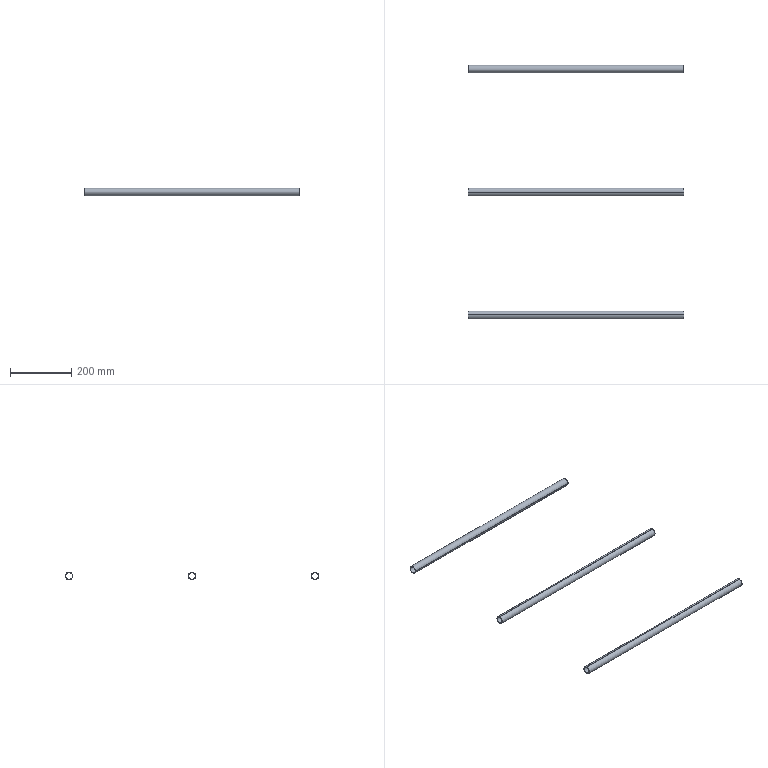Part | STEP file | E3-粉仓护栏10栏杆_Default<As Machined> | 3 solids | 18 faces | box 702.5 x 825 x 25 mm | volume 233387 mm3 | cylinder 12 | plane 6 | commonest cylinder face diameters 22 x6 25 x6
STEP:
#1=CARTESIAN_POINT('',(0.,0.,0.));
#2=DIRECTION('',(0.,0.,1.));
#3=DIRECTION('',(1.,0.,0.));
#4=AXIS2_PLACEMENT_3D('',#1,#2,#3);
#5=CARTESIAN_POINT('',(-702.5,0.,12.5));
#6=VERTEX_POINT('',#5);
#7=CARTESIAN_POINT('',(-702.5,0.,-12.5));
#8=VERTEX_POINT('',#7);
#9=CARTESIAN_POINT('',(-702.5,0.,0.));
#10=DIRECTION('',(1.,0.,0.));
#11=DIRECTION('',(0.,-1.,0.));
#12=AXIS2_PLACEMENT_3D('',#9,#10,#11);
#13=CIRCLE('',#12,12.5);
#14=CARTESIAN_POINT('',(-702.5,0.,0.));
#15=DIRECTION('',(1.,0.,0.));
#16=DIRECTION('',(0.,0.,1.));
#17=AXIS2_PLACEMENT_3D('',#14,#15,#16);
#18=CYLINDRICAL_SURFACE('',#17,12.5);
#19=CARTESIAN_POINT('',(-4.712,0.));
#20=DIRECTION('',(1.,0.));
#21=VECTOR('',#20,1.);
#22=LINE('',#19,#21);
#23=(GEOMETRIC_REPRESENTATION_CONTEXT(2)PARAMETRIC_REPRESENTATION_CONTEXT()REPRESENTATION_CONTEXT('',''));
#24=DEFINITIONAL_REPRESENTATION('',(#22),#23);
#25=PCURVE('',#18,#24);
#26=CARTESIAN_POINT('',(-702.5,0.,0.));
#27=DIRECTION('',(-1.,0.,0.));
#28=DIRECTION('',(0.,-1.,0.));
#29=AXIS2_PLACEMENT_3D('',#26,#27,#28);
#30=PLANE('',#29);
#31=CARTESIAN_POINT('',(12.5,0.));
#32=CARTESIAN_POINT('',(12.5,-21.651));
#33=CARTESIAN_POINT('',(-6.25,-10.825));
#34=CARTESIAN_POINT('',(-25.,0.));
#35=CARTESIAN_POINT('',(-6.25,10.825));
#36=CARTESIAN_POINT('',(12.5,21.651));
#37=CARTESIAN_POINT('',(12.5,0.));
#38=(BOUNDED_CURVE()B_SPLINE_CURVE(2,(#31,#32,#33,#34,#35,#36,#37),.UNSPECIFIED.,.T.,.F.)B_SPLINE_CURVE_WITH_KNOTS((1,2,2,2,2,1),(-2.094,0.,2.094,4.189,6.283,8.378),.UNSPECIFIED.)CURVE()GEOMETRIC_REPRESENTATION_ITEM()RATIONAL_B_SPLINE_CURVE((1.,0.5,1.,0.5,1.,0.5,1.))REPRESENTATION_ITEM(''));
#39=(GEOMETRIC_REPRESENTATION_CONTEXT(2)PARAMETRIC_REPRESENTATION_CONTEXT()REPRESENTATION_CONTEXT('',''));
#40=DEFINITIONAL_REPRESENTATION('',(#38),#39);
#41=PCURVE('',#30,#40);
#42=SURFACE_CURVE('',#13,(#25,#41),.PCURVE_S1.);
#43=EDGE_CURVE('',#6,#8,#42,.T.);
#44=ORIENTED_EDGE('',*,*,#43,.T.);
#45=CARTESIAN_POINT('',(0.,0.,-12.5));
#46=VERTEX_POINT('',#45);
#47=CARTESIAN_POINT('',(-702.5,0.,-12.5));
#48=DIRECTION('',(1.,0.,0.));
#49=VECTOR('',#48,1.);
#50=LINE('',#47,#49);
#51=CARTESIAN_POINT('',(3.142,0.));
#52=DIRECTION('',(0.,1.));
#53=VECTOR('',#52,1.);
#54=LINE('',#51,#53);
#55=(GEOMETRIC_REPRESENTATION_CONTEXT(2)PARAMETRIC_REPRESENTATION_CONTEXT()REPRESENTATION_CONTEXT('',''));
#56=DEFINITIONAL_REPRESENTATION('',(#54),#55);
#57=PCURVE('',#18,#56);
#58=CARTESIAN_POINT('',(-702.5,0.,0.));
#59=DIRECTION('',(1.,0.,0.));
#60=DIRECTION('',(0.,0.,1.));
#61=AXIS2_PLACEMENT_3D('',#58,#59,#60);
#62=CYLINDRICAL_SURFACE('',#61,12.5);
#63=CARTESIAN_POINT('',(3.142,0.));
#64=DIRECTION('',(0.,1.));
#65=VECTOR('',#64,1.);
#66=LINE('',#63,#65);
#67=(GEOMETRIC_REPRESENTATION_CONTEXT(2)PARAMETRIC_REPRESENTATION_CONTEXT()REPRESENTATION_CONTEXT('',''));
#68=DEFINITIONAL_REPRESENTATION('',(#66),#67);
#69=PCURVE('',#62,#68);
#70=SURFACE_CURVE('',#50,(#57,#69),.PCURVE_S1.);
#71=EDGE_CURVE('',#8,#46,#70,.T.);
#72=ORIENTED_EDGE('',*,*,#71,.T.);
#73=CARTESIAN_POINT('',(0.,0.,12.5));
#74=VERTEX_POINT('',#73);
#75=CARTESIAN_POINT('',(0.,0.,0.));
#76=DIRECTION('',(1.,0.,0.));
#77=DIRECTION('',(0.,-1.,0.));
#78=AXIS2_PLACEMENT_3D('',#75,#76,#77);
#79=CIRCLE('',#78,12.5);
#80=CARTESIAN_POINT('',(-4.712,702.5));
#81=DIRECTION('',(1.,0.));
#82=VECTOR('',#81,1.);
#83=LINE('',#80,#82);
#84=(GEOMETRIC_REPRESENTATION_CONTEXT(2)PARAMETRIC_REPRESENTATION_CONTEXT()REPRESENTATION_CONTEXT('',''));
#85=DEFINITIONAL_REPRESENTATION('',(#83),#84);
#86=PCURVE('',#18,#85);
#87=CARTESIAN_POINT('',(0.,0.,0.));
#88=DIRECTION('',(-1.,0.,0.));
#89=DIRECTION('',(0.,-1.,0.));
#90=AXIS2_PLACEMENT_3D('',#87,#88,#89);
#91=PLANE('',#90);
#92=CARTESIAN_POINT('',(12.5,0.));
#93=CARTESIAN_POINT('',(12.5,-21.651));
#94=CARTESIAN_POINT('',(-6.25,-10.825));
#95=CARTESIAN_POINT('',(-25.,0.));
#96=CARTESIAN_POINT('',(-6.25,10.825));
#97=CARTESIAN_POINT('',(12.5,21.651));
#98=CARTESIAN_POINT('',(12.5,0.));
#99=(BOUNDED_CURVE()B_SPLINE_CURVE(2,(#92,#93,#94,#95,#96,#97,#98),.UNSPECIFIED.,.T.,.F.)B_SPLINE_CURVE_WITH_KNOTS((1,2,2,2,2,1),(-2.094,0.,2.094,4.189,6.283,8.378),.UNSPECIFIED.)CURVE()GEOMETRIC_REPRESENTATION_ITEM()RATIONAL_B_SPLINE_CURVE((1.,0.5,1.,0.5,1.,0.5,1.))REPRESENTATION_ITEM(''));
#100=(GEOMETRIC_REPRESENTATION_CONTEXT(2)PARAMETRIC_REPRESENTATION_CONTEXT()REPRESENTATION_CONTEXT('',''));
#101=DEFINITIONAL_REPRESENTATION('',(#99),#100);
#102=PCURVE('',#91,#101);
#103=SURFACE_CURVE('',#79,(#86,#102),.PCURVE_S1.);
#104=EDGE_CURVE('',#74,#46,#103,.T.);
#105=ORIENTED_EDGE('',*,*,#104,.F.);
#106=CARTESIAN_POINT('',(-702.5,0.,12.5));
#107=DIRECTION('',(1.,0.,0.));
#108=VECTOR('',#107,1.);
#109=LINE('',#106,#108);
#110=CARTESIAN_POINT('',(0.,0.));
#111=DIRECTION('',(0.,1.));
#112=VECTOR('',#111,1.);
#113=LINE('',#110,#112);
#114=(GEOMETRIC_REPRESENTATION_CONTEXT(2)PARAMETRIC_REPRESENTATION_CONTEXT()REPRESENTATION_CONTEXT('',''));
#115=DEFINITIONAL_REPRESENTATION('',(#113),#114);
#116=PCURVE('',#18,#115);
#117=CARTESIAN_POINT('',(6.283,0.));
#118=DIRECTION('',(0.,1.));
#119=VECTOR('',#118,1.);
#120=LINE('',#117,#119);
#121=(GEOMETRIC_REPRESENTATION_CONTEXT(2)PARAMETRIC_REPRESENTATION_CONTEXT()REPRESENTATION_CONTEXT('',''));
#122=DEFINITIONAL_REPRESENTATION('',(#120),#121);
#123=PCURVE('',#62,#122);
#124=SURFACE_CURVE('',#109,(#116,#123),.PCURVE_S1.);
#125=EDGE_CURVE('',#6,#74,#124,.T.);
#126=ORIENTED_EDGE('',*,*,#125,.F.);
#127=EDGE_LOOP('',(#44,#72,#105,#126));
#128=FACE_BOUND('',#127,.T.);
#129=ADVANCED_FACE('',(#128),#18,.T.);
#130=CARTESIAN_POINT('',(-702.5,0.,11.));
#131=VERTEX_POINT('',#130);
#132=CARTESIAN_POINT('',(0.,0.,11.));
#133=VERTEX_POINT('',#132);
#134=CARTESIAN_POINT('',(-702.5,0.,11.));
#135=DIRECTION('',(1.,0.,0.));
#136=VECTOR('',#135,1.);
#137=LINE('',#134,#136);
#138=CARTESIAN_POINT('',(-702.5,0.,0.));
#139=DIRECTION('',(1.,0.,0.));
#140=DIRECTION('',(0.,0.,1.));
#141=AXIS2_PLACEMENT_3D('',#138,#139,#140);
#142=CYLINDRICAL_SURFACE('',#141,11.);
#143=CARTESIAN_POINT('',(6.283,0.));
#144=DIRECTION('',(0.,1.));
#145=VECTOR('',#144,1.);
#146=LINE('',#143,#145);
#147=(GEOMETRIC_REPRESENTATION_CONTEXT(2)PARAMETRIC_REPRESENTATION_CONTEXT()REPRESENTATION_CONTEXT('',''));
#148=DEFINITIONAL_REPRESENTATION('',(#146),#147);
#149=PCURVE('',#142,#148);
#150=CARTESIAN_POINT('',(-702.5,0.,0.));
#151=DIRECTION('',(1.,0.,0.));
#152=DIRECTION('',(0.,0.,1.));
#153=AXIS2_PLACEMENT_3D('',#150,#151,#152);
#154=CYLINDRICAL_SURFACE('',#153,11.);
#155=CARTESIAN_POINT('',(0.,0.));
#156=DIRECTION('',(0.,1.));
#157=VECTOR('',#156,1.);
#158=LINE('',#155,#157);
#159=(GEOMETRIC_REPRESENTATION_CONTEXT(2)PARAMETRIC_REPRESENTATION_CONTEXT()REPRESENTATION_CONTEXT('',''));
#160=DEFINITIONAL_REPRESENTATION('',(#158),#159);
#161=PCURVE('',#154,#160);
#162=SURFACE_CURVE('',#137,(#149,#161),.PCURVE_S1.);
#163=EDGE_CURVE('',#131,#133,#162,.T.);
#164=ORIENTED_EDGE('',*,*,#163,.T.);
#165=CARTESIAN_POINT('',(0.,0.,-11.));
#166=VERTEX_POINT('',#165);
#167=CARTESIAN_POINT('',(0.,0.,0.));
#168=DIRECTION('',(1.,0.,0.));
#169=DIRECTION('',(0.,-1.,0.));
#170=AXIS2_PLACEMENT_3D('',#167,#168,#169);
#171=CIRCLE('',#170,11.);
#172=CARTESIAN_POINT('',(1.571,702.5));
#173=DIRECTION('',(1.,0.));
#174=VECTOR('',#173,1.);
#175=LINE('',#172,#174);
#176=(GEOMETRIC_REPRESENTATION_CONTEXT(2)PARAMETRIC_REPRESENTATION_CONTEXT()REPRESENTATION_CONTEXT('',''));
#177=DEFINITIONAL_REPRESENTATION('',(#175),#176);
#178=PCURVE('',#142,#177);
#179=CARTESIAN_POINT('',(11.,0.));
#180=CARTESIAN_POINT('',(11.,-19.053));
#181=CARTESIAN_POINT('',(-5.5,-9.526));
#182=CARTESIAN_POINT('',(-22.,0.));
#183=CARTESIAN_POINT('',(-5.5,9.526));
#184=CARTESIAN_POINT('',(11.,19.053));
#185=CARTESIAN_POINT('',(11.,0.));
#186=(BOUNDED_CURVE()B_SPLINE_CURVE(2,(#179,#180,#181,#182,#183,#184,#185),.UNSPECIFIED.,.T.,.F.)B_SPLINE_CURVE_WITH_KNOTS((1,2,2,2,2,1),(-2.094,0.,2.094,4.189,6.283,8.378),.UNSPECIFIED.)CURVE()GEOMETRIC_REPRESENTATION_ITEM()RATIONAL_B_SPLINE_CURVE((1.,0.5,1.,0.5,1.,0.5,1.))REPRESENTATION_ITEM(''));
#187=(GEOMETRIC_REPRESENTATION_CONTEXT(2)PARAMETRIC_REPRESENTATION_CONTEXT()REPRESENTATION_CONTEXT('',''));
#188=DEFINITIONAL_REPRESENTATION('',(#186),#187);
#189=PCURVE('',#91,#188);
#190=SURFACE_CURVE('',#171,(#178,#189),.PCURVE_S1.);
#191=EDGE_CURVE('',#166,#133,#190,.T.);
#192=ORIENTED_EDGE('',*,*,#191,.F.);
#193=CARTESIAN_POINT('',(-702.5,0.,-11.));
#194=VERTEX_POINT('',#193);
#195=CARTESIAN_POINT('',(-702.5,0.,-11.));
#196=DIRECTION('',(1.,0.,0.));
#197=VECTOR('',#196,1.);
#198=LINE('',#195,#197);
#199=CARTESIAN_POINT('',(3.142,0.));
#200=DIRECTION('',(0.,1.));
#201=VECTOR('',#200,1.);
#202=LINE('',#199,#201);
#203=(GEOMETRIC_REPRESENTATION_CONTEXT(2)PARAMETRIC_REPRESENTATION_CONTEXT()REPRESENTATION_CONTEXT('',''));
#204=DEFINITIONAL_REPRESENTATION('',(#202),#203);
#205=PCURVE('',#142,#204);
#206=CARTESIAN_POINT('',(3.142,0.));
#207=DIRECTION('',(0.,1.));
#208=VECTOR('',#207,1.);
#209=LINE('',#206,#208);
#210=(GEOMETRIC_REPRESENTATION_CONTEXT(2)PARAMETRIC_REPRESENTATION_CONTEXT()REPRESENTATION_CONTEXT('',''));
#211=DEFINITIONAL_REPRESENTATION('',(#209),#210);
#212=PCURVE('',#154,#211);
#213=SURFACE_CURVE('',#198,(#205,#212),.PCURVE_S1.);
#214=EDGE_CURVE('',#194,#166,#213,.T.);
#215=ORIENTED_EDGE('',*,*,#214,.F.);
#216=CARTESIAN_POINT('',(-702.5,0.,0.));
#217=DIRECTION('',(1.,0.,0.));
#218=DIRECTION('',(0.,-1.,0.));
#219=AXIS2_PLACEMENT_3D('',#216,#217,#218);
#220=CIRCLE('',#219,11.);
#221=CARTESIAN_POINT('',(1.571,0.));
#222=DIRECTION('',(1.,0.));
#223=VECTOR('',#222,1.);
#224=LINE('',#221,#223);
#225=(GEOMETRIC_REPRESENTATION_CONTEXT(2)PARAMETRIC_REPRESENTATION_CONTEXT()REPRESENTATION_CONTEXT('',''));
#226=DEFINITIONAL_REPRESENTATION('',(#224),#225);
#227=PCURVE('',#142,#226);
#228=CARTESIAN_POINT('',(11.,0.));
#229=CARTESIAN_POINT('',(11.,-19.053));
#230=CARTESIAN_POINT('',(-5.5,-9.526));
#231=CARTESIAN_POINT('',(-22.,0.));
#232=CARTESIAN_POINT('',(-5.5,9.526));
#233=CARTESIAN_POINT('',(11.,19.053));
#234=CARTESIAN_POINT('',(11.,0.));
#235=(BOUNDED_CURVE()B_SPLINE_CURVE(2,(#228,#229,#230,#231,#232,#233,#234),.UNSPECIFIED.,.T.,.F.)B_SPLINE_CURVE_WITH_KNOTS((1,2,2,2,2,1),(-2.094,0.,2.094,4.189,6.283,8.378),.UNSPECIFIED.)CURVE()GEOMETRIC_REPRESENTATION_ITEM()RATIONAL_B_SPLINE_CURVE((1.,0.5,1.,0.5,1.,0.5,1.))REPRESENTATION_ITEM(''));
#236=(GEOMETRIC_REPRESENTATION_CONTEXT(2)PARAMETRIC_REPRESENTATION_CONTEXT()REPRESENTATION_CONTEXT('',''));
#237=DEFINITIONAL_REPRESENTATION('',(#235),#236);
#238=PCURVE('',#30,#237);
#239=SURFACE_CURVE('',#220,(#227,#238),.PCURVE_S1.);
#240=EDGE_CURVE('',#194,#131,#239,.T.);
#241=ORIENTED_EDGE('',*,*,#240,.T.);
#242=EDGE_LOOP('',(#164,#192,#215,#241));
#243=FACE_BOUND('',#242,.F.);
#244=ADVANCED_FACE('',(#243),#142,.F.);
#245=CARTESIAN_POINT('',(0.,0.,0.));
#246=DIRECTION('',(1.,0.,0.));
#247=DIRECTION('',(0.,-1.,0.));
#248=AXIS2_PLACEMENT_3D('',#245,#246,#247);
#249=CIRCLE('',#248,11.);
#250=CARTESIAN_POINT('',(-4.712,702.5));
#251=DIRECTION('',(1.,0.));
#252=VECTOR('',#251,1.);
#253=LINE('',#250,#252);
#254=(GEOMETRIC_REPRESENTATION_CONTEXT(2)PARAMETRIC_REPRESENTATION_CONTEXT()REPRESENTATION_CONTEXT('',''));
#255=DEFINITIONAL_REPRESENTATION('',(#253),#254);
#256=PCURVE('',#154,#255);
#257=CARTESIAN_POINT('',(11.,0.));
#258=CARTESIAN_POINT('',(11.,-19.053));
#259=CARTESIAN_POINT('',(-5.5,-9.526));
#260=CARTESIAN_POINT('',(-22.,0.));
#261=CARTESIAN_POINT('',(-5.5,9.526));
#262=CARTESIAN_POINT('',(11.,19.053));
#263=CARTESIAN_POINT('',(11.,0.));
#264=(BOUNDED_CURVE()B_SPLINE_CURVE(2,(#257,#258,#259,#260,#261,#262,#263),.UNSPECIFIED.,.T.,.F.)B_SPLINE_CURVE_WITH_KNOTS((1,2,2,2,2,1),(-2.094,0.,2.094,4.189,6.283,8.378),.UNSPECIFIED.)CURVE()GEOMETRIC_REPRESENTATION_ITEM()RATIONAL_B_SPLINE_CURVE((1.,0.5,1.,0.5,1.,0.5,1.))REPRESENTATION_ITEM(''));
#265=(GEOMETRIC_REPRESENTATION_CONTEXT(2)PARAMETRIC_REPRESENTATION_CONTEXT()REPRESENTATION_CONTEXT('',''));
#266=DEFINITIONAL_REPRESENTATION('',(#264),#265);
#267=PCURVE('',#91,#266);
#268=SURFACE_CURVE('',#249,(#256,#267),.PCURVE_S1.);
#269=EDGE_CURVE('',#133,#166,#268,.T.);
#270=ORIENTED_EDGE('',*,*,#269,.F.);
#271=ORIENTED_EDGE('',*,*,#163,.F.);
#272=CARTESIAN_POINT('',(-702.5,0.,0.));
#273=DIRECTION('',(1.,0.,0.));
#274=DIRECTION('',(0.,-1.,0.));
#275=AXIS2_PLACEMENT_3D('',#272,#273,#274);
#276=CIRCLE('',#275,11.);
#277=CARTESIAN_POINT('',(-4.712,0.));
#278=DIRECTION('',(1.,0.));
#279=VECTOR('',#278,1.);
#280=LINE('',#277,#279);
#281=(GEOMETRIC_REPRESENTATION_CONTEXT(2)PARAMETRIC_REPRESENTATION_CONTEXT()REPRESENTATION_CONTEXT('',''));
#282=DEFINITIONAL_REPRESENTATION('',(#280),#281);
#283=PCURVE('',#154,#282);
#284=CARTESIAN_POINT('',(11.,0.));
#285=CARTESIAN_POINT('',(11.,-19.053));
#286=CARTESIAN_POINT('',(-5.5,-9.526));
#287=CARTESIAN_POINT('',(-22.,0.));
#288=CARTESIAN_POINT('',(-5.5,9.526));
#289=CARTESIAN_POINT('',(11.,19.053));
#290=CARTESIAN_POINT('',(11.,0.));
#291=(BOUNDED_CURVE()B_SPLINE_CURVE(2,(#284,#285,#286,#287,#288,#289,#290),.UNSPECIFIED.,.T.,.F.)B_SPLINE_CURVE_WITH_KNOTS((1,2,2,2,2,1),(-2.094,0.,2.094,4.189,6.283,8.378),.UNSPECIFIED.)CURVE()GEOMETRIC_REPRESENTATION_ITEM()RATIONAL_B_SPLINE_CURVE((1.,0.5,1.,0.5,1.,0.5,1.))REPRESENTATION_ITEM(''));
#292=(GEOMETRIC_REPRESENTATION_CONTEXT(2)PARAMETRIC_REPRESENTATION_CONTEXT()REPRESENTATION_CONTEXT('',''));
#293=DEFINITIONAL_REPRESENTATION('',(#291),#292);
#294=PCURVE('',#30,#293);
#295=SURFACE_CURVE('',#276,(#283,#294),.PCURVE_S1.);
#296=EDGE_CURVE('',#131,#194,#295,.T.);
#297=ORIENTED_EDGE('',*,*,#296,.T.);
#298=ORIENTED_EDGE('',*,*,#214,.T.);
#299=EDGE_LOOP('',(#270,#271,#297,#298));
#300=FACE_BOUND('',#299,.F.);
#301=ADVANCED_FACE('',(#300),#154,.F.);
#302=ORIENTED_EDGE('',*,*,#71,.F.);
#303=CARTESIAN_POINT('',(-702.5,0.,0.));
#304=DIRECTION('',(1.,0.,0.));
#305=DIRECTION('',(0.,-1.,0.));
#306=AXIS2_PLACEMENT_3D('',#303,#304,#305);
#307=CIRCLE('',#306,12.5);
#308=CARTESIAN_POINT('',(1.571,0.));
#309=DIRECTION('',(1.,0.));
#310=VECTOR('',#309,1.);
#311=LINE('',#308,#310);
#312=(GEOMETRIC_REPRESENTATION_CONTEXT(2)PARAMETRIC_REPRESENTATION_CONTEXT()REPRESENTATION_CONTEXT('',''));
#313=DEFINITIONAL_REPRESENTATION('',(#311),#312);
#314=PCURVE('',#62,#313);
#315=CARTESIAN_POINT('',(12.5,0.));
#316=CARTESIAN_POINT('',(12.5,-21.651));
#317=CARTESIAN_POINT('',(-6.25,-10.825));
#318=CARTESIAN_POINT('',(-25.,0.));
#319=CARTESIAN_POINT('',(-6.25,10.825));
#320=CARTESIAN_POINT('',(12.5,21.651));
#321=CARTESIAN_POINT('',(12.5,0.));
#322=(BOUNDED_CURVE()B_SPLINE_CURVE(2,(#315,#316,#317,#318,#319,#320,#321),.UNSPECIFIED.,.T.,.F.)B_SPLINE_CURVE_WITH_KNOTS((1,2,2,2,2,1),(-2.094,0.,2.094,4.189,6.283,8.378),.UNSPECIFIED.)CURVE()GEOMETRIC_REPRESENTATION_ITEM()RATIONAL_B_SPLINE_CURVE((1.,0.5,1.,0.5,1.,0.5,1.))REPRESENTATION_ITEM(''));
#323=(GEOMETRIC_REPRESENTATION_CONTEXT(2)PARAMETRIC_REPRESENTATION_CONTEXT()REPRESENTATION_CONTEXT('',''));
#324=DEFINITIONAL_REPRESENTATION('',(#322),#323);
#325=PCURVE('',#30,#324);
#326=SURFACE_CURVE('',#307,(#314,#325),.PCURVE_S1.);
#327=EDGE_CURVE('',#8,#6,#326,.T.);
#328=ORIENTED_EDGE('',*,*,#327,.T.);
#329=ORIENTED_EDGE('',*,*,#125,.T.);
#330=CARTESIAN_POINT('',(0.,0.,0.));
#331=DIRECTION('',(1.,0.,0.));
#332=DIRECTION('',(0.,-1.,0.));
#333=AXIS2_PLACEMENT_3D('',#330,#331,#332);
#334=CIRCLE('',#333,12.5);
#335=CARTESIAN_POINT('',(1.571,702.5));
#336=DIRECTION('',(1.,0.));
#337=VECTOR('',#336,1.);
#338=LINE('',#335,#337);
#339=(GEOMETRIC_REPRESENTATION_CONTEXT(2)PARAMETRIC_REPRESENTATION_CONTEXT()REPRESENTATION_CONTEXT('',''));
#340=DEFINITIONAL_REPRESENTATION('',(#338),#339);
#341=PCURVE('',#62,#340);
#342=CARTESIAN_POINT('',(12.5,0.));
#343=CARTESIAN_POINT('',(12.5,-21.651));
#344=CARTESIAN_POINT('',(-6.25,-10.825));
#345=CARTESIAN_POINT('',(-25.,0.));
#346=CARTESIAN_POINT('',(-6.25,10.825));
#347=CARTESIAN_POINT('',(12.5,21.651));
#348=CARTESIAN_POINT('',(12.5,0.));
#349=(BOUNDED_CURVE()B_SPLINE_CURVE(2,(#342,#343,#344,#345,#346,#347,#348),.UNSPECIFIED.,.T.,.F.)B_SPLINE_CURVE_WITH_KNOTS((1,2,2,2,2,1),(-2.094,0.,2.094,4.189,6.283,8.378),.UNSPECIFIED.)CURVE()GEOMETRIC_REPRESENTATION_ITEM()RATIONAL_B_SPLINE_CURVE((1.,0.5,1.,0.5,1.,0.5,1.))REPRESENTATION_ITEM(''));
#350=(GEOMETRIC_REPRESENTATION_CONTEXT(2)PARAMETRIC_REPRESENTATION_CONTEXT()REPRESENTATION_CONTEXT('',''));
#351=DEFINITIONAL_REPRESENTATION('',(#349),#350);
#352=PCURVE('',#91,#351);
#353=SURFACE_CURVE('',#334,(#341,#352),.PCURVE_S1.);
#354=EDGE_CURVE('',#46,#74,#353,.T.);
#355=ORIENTED_EDGE('',*,*,#354,.F.);
#356=EDGE_LOOP('',(#302,#328,#329,#355));
#357=FACE_BOUND('',#356,.T.);
#358=ADVANCED_FACE('',(#357),#62,.T.);
#359=ORIENTED_EDGE('',*,*,#296,.T.);
#360=ORIENTED_EDGE('',*,*,#240,.T.);
#361=EDGE_LOOP('',(#359,#360));
#362=FACE_BOUND('',#361,.T.);
#363=ORIENTED_EDGE('',*,*,#43,.F.);
#364=ORIENTED_EDGE('',*,*,#327,.F.);
#365=EDGE_LOOP('',(#363,#364));
#366=FACE_BOUND('',#365,.T.);
#367=ADVANCED_FACE('',(#362,#366),#30,.T.);
#368=ORIENTED_EDGE('',*,*,#269,.F.);
#369=ORIENTED_EDGE('',*,*,#191,.F.);
#370=EDGE_LOOP('',(#368,#369));
#371=FACE_BOUND('',#370,.T.);
#372=ORIENTED_EDGE('',*,*,#104,.T.);
#373=ORIENTED_EDGE('',*,*,#354,.T.);
#374=EDGE_LOOP('',(#372,#373));
#375=FACE_BOUND('',#374,.T.);
#376=ADVANCED_FACE('',(#371,#375),#91,.F.);
#377=CLOSED_SHELL('',(#129,#244,#301,#358,#367,#376));
#378=MANIFOLD_SOLID_BREP('',#377);
#379=CARTESIAN_POINT('',(-702.5,812.5,0.));
#380=VERTEX_POINT('',#379);
#381=CARTESIAN_POINT('',(-702.5,787.5,0.));
#382=VERTEX_POINT('',#381);
#383=CARTESIAN_POINT('',(-702.5,800.,0.));
#384=DIRECTION('',(1.,0.,0.));
#385=DIRECTION('',(0.,-1.,0.));
#386=AXIS2_PLACEMENT_3D('',#383,#384,#385);
#387=CIRCLE('',#386,12.5);
#388=CARTESIAN_POINT('',(-702.5,800.,0.));
#389=DIRECTION('',(1.,0.,0.));
#390=DIRECTION('',(0.,1.,0.));
#391=AXIS2_PLACEMENT_3D('',#388,#389,#390);
#392=CYLINDRICAL_SURFACE('',#391,12.5);
#393=CARTESIAN_POINT('',(-3.142,0.));
#394=DIRECTION('',(1.,0.));
#395=VECTOR('',#394,1.);
#396=LINE('',#393,#395);
#397=(GEOMETRIC_REPRESENTATION_CONTEXT(2)PARAMETRIC_REPRESENTATION_CONTEXT()REPRESENTATION_CONTEXT('',''));
#398=DEFINITIONAL_REPRESENTATION('',(#396),#397);
#399=PCURVE('',#392,#398);
#400=CARTESIAN_POINT('',(-702.5,800.,0.));
#401=DIRECTION('',(-1.,0.,0.));
#402=DIRECTION('',(0.,-1.,0.));
#403=AXIS2_PLACEMENT_3D('',#400,#401,#402);
#404=PLANE('',#403);
#405=CARTESIAN_POINT('',(12.5,0.));
#406=CARTESIAN_POINT('',(12.5,-21.651));
#407=CARTESIAN_POINT('',(-6.25,-10.825));
#408=CARTESIAN_POINT('',(-25.,0.));
#409=CARTESIAN_POINT('',(-6.25,10.825));
#410=CARTESIAN_POINT('',(12.5,21.651));
#411=CARTESIAN_POINT('',(12.5,0.));
#412=(BOUNDED_CURVE()B_SPLINE_CURVE(2,(#405,#406,#407,#408,#409,#410,#411),.UNSPECIFIED.,.T.,.F.)B_SPLINE_CURVE_WITH_KNOTS((1,2,2,2,2,1),(-2.094,0.,2.094,4.189,6.283,8.378),.UNSPECIFIED.)CURVE()GEOMETRIC_REPRESENTATION_ITEM()RATIONAL_B_SPLINE_CURVE((1.,0.5,1.,0.5,1.,0.5,1.))REPRESENTATION_ITEM(''));
#413=(GEOMETRIC_REPRESENTATION_CONTEXT(2)PARAMETRIC_REPRESENTATION_CONTEXT()REPRESENTATION_CONTEXT('',''));
#414=DEFINITIONAL_REPRESENTATION('',(#412),#413);
#415=PCURVE('',#404,#414);
#416=SURFACE_CURVE('',#387,(#399,#415),.PCURVE_S1.);
#417=EDGE_CURVE('',#380,#382,#416,.T.);
#418=ORIENTED_EDGE('',*,*,#417,.T.);
#419=CARTESIAN_POINT('',(0.,787.5,0.));
#420=VERTEX_POINT('',#419);
#421=CARTESIAN_POINT('',(-702.5,787.5,0.));
#422=DIRECTION('',(1.,0.,0.));
#423=VECTOR('',#422,1.);
#424=LINE('',#421,#423);
#425=CARTESIAN_POINT('',(3.142,0.));
#426=DIRECTION('',(0.,1.));
#427=VECTOR('',#426,1.);
#428=LINE('',#425,#427);
#429=(GEOMETRIC_REPRESENTATION_CONTEXT(2)PARAMETRIC_REPRESENTATION_CONTEXT()REPRESENTATION_CONTEXT('',''));
#430=DEFINITIONAL_REPRESENTATION('',(#428),#429);
#431=PCURVE('',#392,#430);
#432=CARTESIAN_POINT('',(-702.5,800.,0.));
#433=DIRECTION('',(1.,0.,0.));
#434=DIRECTION('',(0.,1.,0.));
#435=AXIS2_PLACEMENT_3D('',#432,#433,#434);
#436=CYLINDRICAL_SURFACE('',#435,12.5);
#437=CARTESIAN_POINT('',(3.142,0.));
#438=DIRECTION('',(0.,1.));
#439=VECTOR('',#438,1.);
#440=LINE('',#437,#439);
#441=(GEOMETRIC_REPRESENTATION_CONTEXT(2)PARAMETRIC_REPRESENTATION_CONTEXT()REPRESENTATION_CONTEXT('',''));
#442=DEFINITIONAL_REPRESENTATION('',(#440),#441);
#443=PCURVE('',#436,#442);
#444=SURFACE_CURVE('',#424,(#431,#443),.PCURVE_S1.);
#445=EDGE_CURVE('',#382,#420,#444,.T.);
#446=ORIENTED_EDGE('',*,*,#445,.T.);
#447=CARTESIAN_POINT('',(0.,812.5,0.));
#448=VERTEX_POINT('',#447);
#449=CARTESIAN_POINT('',(0.,800.,0.));
#450=DIRECTION('',(1.,0.,0.));
#451=DIRECTION('',(0.,-1.,0.));
#452=AXIS2_PLACEMENT_3D('',#449,#450,#451);
#453=CIRCLE('',#452,12.5);
#454=CARTESIAN_POINT('',(-3.142,702.5));
#455=DIRECTION('',(1.,0.));
#456=VECTOR('',#455,1.);
#457=LINE('',#454,#456);
#458=(GEOMETRIC_REPRESENTATION_CONTEXT(2)PARAMETRIC_REPRESENTATION_CONTEXT()REPRESENTATION_CONTEXT('',''));
#459=DEFINITIONAL_REPRESENTATION('',(#457),#458);
#460=PCURVE('',#392,#459);
#461=CARTESIAN_POINT('',(0.,800.,0.));
#462=DIRECTION('',(-1.,0.,0.));
#463=DIRECTION('',(0.,-1.,0.));
#464=AXIS2_PLACEMENT_3D('',#461,#462,#463);
#465=PLANE('',#464);
#466=CARTESIAN_POINT('',(12.5,0.));
#467=CARTESIAN_POINT('',(12.5,-21.651));
#468=CARTESIAN_POINT('',(-6.25,-10.825));
#469=CARTESIAN_POINT('',(-25.,0.));
#470=CARTESIAN_POINT('',(-6.25,10.825));
#471=CARTESIAN_POINT('',(12.5,21.651));
#472=CARTESIAN_POINT('',(12.5,0.));
#473=(BOUNDED_CURVE()B_SPLINE_CURVE(2,(#466,#467,#468,#469,#470,#471,#472),.UNSPECIFIED.,.T.,.F.)B_SPLINE_CURVE_WITH_KNOTS((1,2,2,2,2,1),(-2.094,0.,2.094,4.189,6.283,8.378),.UNSPECIFIED.)CURVE()GEOMETRIC_REPRESENTATION_ITEM()RATIONAL_B_SPLINE_CURVE((1.,0.5,1.,0.5,1.,0.5,1.))REPRESENTATION_ITEM(''));
#474=(GEOMETRIC_REPRESENTATION_CONTEXT(2)PARAMETRIC_REPRESENTATION_CONTEXT()REPRESENTATION_CONTEXT('',''));
#475=DEFINITIONAL_REPRESENTATION('',(#473),#474);
#476=PCURVE('',#465,#475);
#477=SURFACE_CURVE('',#453,(#460,#476),.PCURVE_S1.);
#478=EDGE_CURVE('',#448,#420,#477,.T.);
#479=ORIENTED_EDGE('',*,*,#478,.F.);
#480=CARTESIAN_POINT('',(-702.5,812.5,0.));
#481=DIRECTION('',(1.,0.,0.));
#482=VECTOR('',#481,1.);
#483=LINE('',#480,#482);
#484=CARTESIAN_POINT('',(0.,0.));
#485=DIRECTION('',(0.,1.));
#486=VECTOR('',#485,1.);
#487=LINE('',#484,#486);
#488=(GEOMETRIC_REPRESENTATION_CONTEXT(2)PARAMETRIC_REPRESENTATION_CONTEXT()REPRESENTATION_CONTEXT('',''));
#489=DEFINITIONAL_REPRESENTATION('',(#487),#488);
#490=PCURVE('',#392,#489);
#491=CARTESIAN_POINT('',(6.283,0.));
#492=DIRECTION('',(0.,1.));
#493=VECTOR('',#492,1.);
#494=LINE('',#491,#493);
#495=(GEOMETRIC_REPRESENTATION_CONTEXT(2)PARAMETRIC_REPRESENTATION_CONTEXT()REPRESENTATION_CONTEXT('',''));
#496=DEFINITIONAL_REPRESENTATION('',(#494),#495);
#497=PCURVE('',#436,#496);
#498=SURFACE_CURVE('',#483,(#490,#497),.PCURVE_S1.);
#499=EDGE_CURVE('',#380,#448,#498,.T.);
#500=ORIENTED_EDGE('',*,*,#499,.F.);
#501=EDGE_LOOP('',(#418,#446,#479,#500));
#502=FACE_BOUND('',#501,.T.);
#503=ADVANCED_FACE('',(#502),#392,.T.);
#504=CARTESIAN_POINT('',(-702.5,811.,0.));
#505=VERTEX_POINT('',#504);
#506=CARTESIAN_POINT('',(0.,811.,0.));
#507=VERTEX_POINT('',#506);
#508=CARTESIAN_POINT('',(-702.5,811.,0.));
#509=DIRECTION('',(1.,0.,0.));
#510=VECTOR('',#509,1.);
#511=LINE('',#508,#510);
#512=CARTESIAN_POINT('',(-702.5,800.,0.));
#513=DIRECTION('',(1.,0.,0.));
#514=DIRECTION('',(0.,1.,0.));
#515=AXIS2_PLACEMENT_3D('',#512,#513,#514);
#516=CYLINDRICAL_SURFACE('',#515,11.);
#517=CARTESIAN_POINT('',(6.283,0.));
#518=DIRECTION('',(0.,1.));
#519=VECTOR('',#518,1.);
#520=LINE('',#517,#519);
#521=(GEOMETRIC_REPRESENTATION_CONTEXT(2)PARAMETRIC_REPRESENTATION_CONTEXT()REPRESENTATION_CONTEXT('',''));
#522=DEFINITIONAL_REPRESENTATION('',(#520),#521);
#523=PCURVE('',#516,#522);
#524=CARTESIAN_POINT('',(-702.5,800.,0.));
#525=DIRECTION('',(1.,0.,0.));
#526=DIRECTION('',(0.,1.,0.));
#527=AXIS2_PLACEMENT_3D('',#524,#525,#526);
#528=CYLINDRICAL_SURFACE('',#527,11.);
#529=CARTESIAN_POINT('',(0.,0.));
#530=DIRECTION('',(0.,1.));
#531=VECTOR('',#530,1.);
#532=LINE('',#529,#531);
#533=(GEOMETRIC_REPRESENTATION_CONTEXT(2)PARAMETRIC_REPRESENTATION_CONTEXT()REPRESENTATION_CONTEXT('',''));
#534=DEFINITIONAL_REPRESENTATION('',(#532),#533);
#535=PCURVE('',#528,#534);
#536=SURFACE_CURVE('',#511,(#523,#535),.PCURVE_S1.);
#537=EDGE_CURVE('',#505,#507,#536,.T.);
#538=ORIENTED_EDGE('',*,*,#537,.T.);
#539=CARTESIAN_POINT('',(0.,789.,0.));
#540=VERTEX_POINT('',#539);
#541=CARTESIAN_POINT('',(0.,800.,0.));
#542=DIRECTION('',(1.,0.,0.));
#543=DIRECTION('',(0.,-1.,0.));
#544=AXIS2_PLACEMENT_3D('',#541,#542,#543);
#545=CIRCLE('',#544,11.);
#546=CARTESIAN_POINT('',(3.142,702.5));
#547=DIRECTION('',(1.,0.));
#548=VECTOR('',#547,1.);
#549=LINE('',#546,#548);
#550=(GEOMETRIC_REPRESENTATION_CONTEXT(2)PARAMETRIC_REPRESENTATION_CONTEXT()REPRESENTATION_CONTEXT('',''));
#551=DEFINITIONAL_REPRESENTATION('',(#549),#550);
#552=PCURVE('',#516,#551);
#553=CARTESIAN_POINT('',(11.,0.));
#554=CARTESIAN_POINT('',(11.,-19.053));
#555=CARTESIAN_POINT('',(-5.5,-9.526));
#556=CARTESIAN_POINT('',(-22.,0.));
#557=CARTESIAN_POINT('',(-5.5,9.526));
#558=CARTESIAN_POINT('',(11.,19.053));
#559=CARTESIAN_POINT('',(11.,0.));
#560=(BOUNDED_CURVE()B_SPLINE_CURVE(2,(#553,#554,#555,#556,#557,#558,#559),.UNSPECIFIED.,.T.,.F.)B_SPLINE_CURVE_WITH_KNOTS((1,2,2,2,2,1),(-2.094,0.,2.094,4.189,6.283,8.378),.UNSPECIFIED.)CURVE()GEOMETRIC_REPRESENTATION_ITEM()RATIONAL_B_SPLINE_CURVE((1.,0.5,1.,0.5,1.,0.5,1.))REPRESENTATION_ITEM(''));
#561=(GEOMETRIC_REPRESENTATION_CONTEXT(2)PARAMETRIC_REPRESENTATION_CONTEXT()REPRESENTATION_CONTEXT('',''));
#562=DEFINITIONAL_REPRESENTATION('',(#560),#561);
#563=PCURVE('',#465,#562);
#564=SURFACE_CURVE('',#545,(#552,#563),.PCURVE_S1.);
#565=EDGE_CURVE('',#540,#507,#564,.T.);
#566=ORIENTED_EDGE('',*,*,#565,.F.);
#567=CARTESIAN_POINT('',(-702.5,789.,0.));
#568=VERTEX_POINT('',#567);
#569=CARTESIAN_POINT('',(-702.5,789.,0.));
#570=DIRECTION('',(1.,0.,0.));
#571=VECTOR('',#570,1.);
#572=LINE('',#569,#571);
#573=CARTESIAN_POINT('',(3.142,0.));
#574=DIRECTION('',(0.,1.));
#575=VECTOR('',#574,1.);
#576=LINE('',#573,#575);
#577=(GEOMETRIC_REPRESENTATION_CONTEXT(2)PARAMETRIC_REPRESENTATION_CONTEXT()REPRESENTATION_CONTEXT('',''));
#578=DEFINITIONAL_REPRESENTATION('',(#576),#577);
#579=PCURVE('',#516,#578);
#580=CARTESIAN_POINT('',(3.142,0.));
#581=DIRECTION('',(0.,1.));
#582=VECTOR('',#581,1.);
#583=LINE('',#580,#582);
#584=(GEOMETRIC_REPRESENTATION_CONTEXT(2)PARAMETRIC_REPRESENTATION_CONTEXT()REPRESENTATION_CONTEXT('',''));
#585=DEFINITIONAL_REPRESENTATION('',(#583),#584);
#586=PCURVE('',#528,#585);
#587=SURFACE_CURVE('',#572,(#579,#586),.PCURVE_S1.);
#588=EDGE_CURVE('',#568,#540,#587,.T.);
#589=ORIENTED_EDGE('',*,*,#588,.F.);
#590=CARTESIAN_POINT('',(-702.5,800.,0.));
#591=DIRECTION('',(1.,0.,0.));
#592=DIRECTION('',(0.,-1.,0.));
#593=AXIS2_PLACEMENT_3D('',#590,#591,#592);
#594=CIRCLE('',#593,11.);
#595=CARTESIAN_POINT('',(3.142,0.));
#596=DIRECTION('',(1.,0.));
#597=VECTOR('',#596,1.);
#598=LINE('',#595,#597);
#599=(GEOMETRIC_REPRESENTATION_CONTEXT(2)PARAMETRIC_REPRESENTATION_CONTEXT()REPRESENTATION_CONTEXT('',''));
#600=DEFINITIONAL_REPRESENTATION('',(#598),#599);
#601=PCURVE('',#516,#600);
#602=CARTESIAN_POINT('',(11.,0.));
#603=CARTESIAN_POINT('',(11.,-19.053));
#604=CARTESIAN_POINT('',(-5.5,-9.526));
#605=CARTESIAN_POINT('',(-22.,0.));
#606=CARTESIAN_POINT('',(-5.5,9.526));
#607=CARTESIAN_POINT('',(11.,19.053));
#608=CARTESIAN_POINT('',(11.,0.));
#609=(BOUNDED_CURVE()B_SPLINE_CURVE(2,(#602,#603,#604,#605,#606,#607,#608),.UNSPECIFIED.,.T.,.F.)B_SPLINE_CURVE_WITH_KNOTS((1,2,2,2,2,1),(-2.094,0.,2.094,4.189,6.283,8.378),.UNSPECIFIED.)CURVE()GEOMETRIC_REPRESENTATION_ITEM()RATIONAL_B_SPLINE_CURVE((1.,0.5,1.,0.5,1.,0.5,1.))REPRESENTATION_ITEM(''));
#610=(GEOMETRIC_REPRESENTATION_CONTEXT(2)PARAMETRIC_REPRESENTATION_CONTEXT()REPRESENTATION_CONTEXT('',''));
#611=DEFINITIONAL_REPRESENTATION('',(#609),#610);
#612=PCURVE('',#404,#611);
#613=SURFACE_CURVE('',#594,(#601,#612),.PCURVE_S1.);
#614=EDGE_CURVE('',#568,#505,#613,.T.);
#615=ORIENTED_EDGE('',*,*,#614,.T.);
#616=EDGE_LOOP('',(#538,#566,#589,#615));
#617=FACE_BOUND('',#616,.F.);
#618=ADVANCED_FACE('',(#617),#516,.F.);
#619=CARTESIAN_POINT('',(0.,800.,0.));
#620=DIRECTION('',(1.,0.,0.));
#621=DIRECTION('',(0.,-1.,0.));
#622=AXIS2_PLACEMENT_3D('',#619,#620,#621);
#623=CIRCLE('',#622,11.);
#624=CARTESIAN_POINT('',(-3.142,702.5));
#625=DIRECTION('',(1.,0.));
#626=VECTOR('',#625,1.);
#627=LINE('',#624,#626);
#628=(GEOMETRIC_REPRESENTATION_CONTEXT(2)PARAMETRIC_REPRESENTATION_CONTEXT()REPRESENTATION_CONTEXT('',''));
#629=DEFINITIONAL_REPRESENTATION('',(#627),#628);
#630=PCURVE('',#528,#629);
#631=CARTESIAN_POINT('',(11.,0.));
#632=CARTESIAN_POINT('',(11.,-19.053));
#633=CARTESIAN_POINT('',(-5.5,-9.526));
#634=CARTESIAN_POINT('',(-22.,0.));
#635=CARTESIAN_POINT('',(-5.5,9.526));
#636=CARTESIAN_POINT('',(11.,19.053));
#637=CARTESIAN_POINT('',(11.,0.));
#638=(BOUNDED_CURVE()B_SPLINE_CURVE(2,(#631,#632,#633,#634,#635,#636,#637),.UNSPECIFIED.,.T.,.F.)B_SPLINE_CURVE_WITH_KNOTS((1,2,2,2,2,1),(-2.094,0.,2.094,4.189,6.283,8.378),.UNSPECIFIED.)CURVE()GEOMETRIC_REPRESENTATION_ITEM()RATIONAL_B_SPLINE_CURVE((1.,0.5,1.,0.5,1.,0.5,1.))REPRESENTATION_ITEM(''));
#639=(GEOMETRIC_REPRESENTATION_CONTEXT(2)PARAMETRIC_REPRESENTATION_CONTEXT()REPRESENTATION_CONTEXT('',''));
#640=DEFINITIONAL_REPRESENTATION('',(#638),#639);
#641=PCURVE('',#465,#640);
#642=SURFACE_CURVE('',#623,(#630,#641),.PCURVE_S1.);
#643=EDGE_CURVE('',#507,#540,#642,.T.);
#644=ORIENTED_EDGE('',*,*,#643,.F.);
#645=ORIENTED_EDGE('',*,*,#537,.F.);
#646=CARTESIAN_POINT('',(-702.5,800.,0.));
#647=DIRECTION('',(1.,0.,0.));
#648=DIRECTION('',(0.,-1.,0.));
#649=AXIS2_PLACEMENT_3D('',#646,#647,#648);
#650=CIRCLE('',#649,11.);
#651=CARTESIAN_POINT('',(-3.142,0.));
#652=DIRECTION('',(1.,0.));
#653=VECTOR('',#652,1.);
#654=LINE('',#651,#653);
#655=(GEOMETRIC_REPRESENTATION_CONTEXT(2)PARAMETRIC_REPRESENTATION_CONTEXT()REPRESENTATION_CONTEXT('',''));
#656=DEFINITIONAL_REPRESENTATION('',(#654),#655);
#657=PCURVE('',#528,#656);
#658=CARTESIAN_POINT('',(11.,0.));
#659=CARTESIAN_POINT('',(11.,-19.053));
#660=CARTESIAN_POINT('',(-5.5,-9.526));
#661=CARTESIAN_POINT('',(-22.,0.));
#662=CARTESIAN_POINT('',(-5.5,9.526));
#663=CARTESIAN_POINT('',(11.,19.053));
#664=CARTESIAN_POINT('',(11.,0.));
#665=(BOUNDED_CURVE()B_SPLINE_CURVE(2,(#658,#659,#660,#661,#662,#663,#664),.UNSPECIFIED.,.T.,.F.)B_SPLINE_CURVE_WITH_KNOTS((1,2,2,2,2,1),(-2.094,0.,2.094,4.189,6.283,8.378),.UNSPECIFIED.)CURVE()GEOMETRIC_REPRESENTATION_ITEM()RATIONAL_B_SPLINE_CURVE((1.,0.5,1.,0.5,1.,0.5,1.))REPRESENTATION_ITEM(''));
#666=(GEOMETRIC_REPRESENTATION_CONTEXT(2)PARAMETRIC_REPRESENTATION_CONTEXT()REPRESENTATION_CONTEXT('',''));
#667=DEFINITIONAL_REPRESENTATION('',(#665),#666);
#668=PCURVE('',#404,#667);
#669=SURFACE_CURVE('',#650,(#657,#668),.PCURVE_S1.);
#670=EDGE_CURVE('',#505,#568,#669,.T.);
#671=ORIENTED_EDGE('',*,*,#670,.T.);
#672=ORIENTED_EDGE('',*,*,#588,.T.);
#673=EDGE_LOOP('',(#644,#645,#671,#672));
#674=FACE_BOUND('',#673,.F.);
#675=ADVANCED_FACE('',(#674),#528,.F.);
#676=ORIENTED_EDGE('',*,*,#445,.F.);
#677=CARTESIAN_POINT('',(-702.5,800.,0.));
#678=DIRECTION('',(1.,0.,0.));
#679=DIRECTION('',(0.,-1.,0.));
#680=AXIS2_PLACEMENT_3D('',#677,#678,#679);
#681=CIRCLE('',#680,12.5);
#682=CARTESIAN_POINT('',(3.142,0.));
#683=DIRECTION('',(1.,0.));
#684=VECTOR('',#683,1.);
#685=LINE('',#682,#684);
#686=(GEOMETRIC_REPRESENTATION_CONTEXT(2)PARAMETRIC_REPRESENTATION_CONTEXT()REPRESENTATION_CONTEXT('',''));
#687=DEFINITIONAL_REPRESENTATION('',(#685),#686);
#688=PCURVE('',#436,#687);
#689=CARTESIAN_POINT('',(12.5,0.));
#690=CARTESIAN_POINT('',(12.5,-21.651));
#691=CARTESIAN_POINT('',(-6.25,-10.825));
#692=CARTESIAN_POINT('',(-25.,0.));
#693=CARTESIAN_POINT('',(-6.25,10.825));
#694=CARTESIAN_POINT('',(12.5,21.651));
#695=CARTESIAN_POINT('',(12.5,0.));
#696=(BOUNDED_CURVE()B_SPLINE_CURVE(2,(#689,#690,#691,#692,#693,#694,#695),.UNSPECIFIED.,.T.,.F.)B_SPLINE_CURVE_WITH_KNOTS((1,2,2,2,2,1),(-2.094,0.,2.094,4.189,6.283,8.378),.UNSPECIFIED.)CURVE()GEOMETRIC_REPRESENTATION_ITEM()RATIONAL_B_SPLINE_CURVE((1.,0.5,1.,0.5,1.,0.5,1.))REPRESENTATION_ITEM(''));
#697=(GEOMETRIC_REPRESENTATION_CONTEXT(2)PARAMETRIC_REPRESENTATION_CONTEXT()REPRESENTATION_CONTEXT('',''));
#698=DEFINITIONAL_REPRESENTATION('',(#696),#697);
#699=PCURVE('',#404,#698);
#700=SURFACE_CURVE('',#681,(#688,#699),.PCURVE_S1.);
#701=EDGE_CURVE('',#382,#380,#700,.T.);
#702=ORIENTED_EDGE('',*,*,#701,.T.);
#703=ORIENTED_EDGE('',*,*,#499,.T.);
#704=CARTESIAN_POINT('',(0.,800.,0.));
#705=DIRECTION('',(1.,0.,0.));
#706=DIRECTION('',(0.,-1.,0.));
#707=AXIS2_PLACEMENT_3D('',#704,#705,#706);
#708=CIRCLE('',#707,12.5);
#709=CARTESIAN_POINT('',(3.142,702.5));
#710=DIRECTION('',(1.,0.));
#711=VECTOR('',#710,1.);
#712=LINE('',#709,#711);
#713=(GEOMETRIC_REPRESENTATION_CONTEXT(2)PARAMETRIC_REPRESENTATION_CONTEXT()REPRESENTATION_CONTEXT('',''));
#714=DEFINITIONAL_REPRESENTATION('',(#712),#713);
#715=PCURVE('',#436,#714);
#716=CARTESIAN_POINT('',(12.5,0.));
#717=CARTESIAN_POINT('',(12.5,-21.651));
#718=CARTESIAN_POINT('',(-6.25,-10.825));
#719=CARTESIAN_POINT('',(-25.,0.));
#720=CARTESIAN_POINT('',(-6.25,10.825));
#721=CARTESIAN_POINT('',(12.5,21.651));
#722=CARTESIAN_POINT('',(12.5,0.));
#723=(BOUNDED_CURVE()B_SPLINE_CURVE(2,(#716,#717,#718,#719,#720,#721,#722),.UNSPECIFIED.,.T.,.F.)B_SPLINE_CURVE_WITH_KNOTS((1,2,2,2,2,1),(-2.094,0.,2.094,4.189,6.283,8.378),.UNSPECIFIED.)CURVE()GEOMETRIC_REPRESENTATION_ITEM()RATIONAL_B_SPLINE_CURVE((1.,0.5,1.,0.5,1.,0.5,1.))REPRESENTATION_ITEM(''));
#724=(GEOMETRIC_REPRESENTATION_CONTEXT(2)PARAMETRIC_REPRESENTATION_CONTEXT()REPRESENTATION_CONTEXT('',''));
#725=DEFINITIONAL_REPRESENTATION('',(#723),#724);
#726=PCURVE('',#465,#725);
#727=SURFACE_CURVE('',#708,(#715,#726),.PCURVE_S1.);
#728=EDGE_CURVE('',#420,#448,#727,.T.);
#729=ORIENTED_EDGE('',*,*,#728,.F.);
#730=EDGE_LOOP('',(#676,#702,#703,#729));
#731=FACE_BOUND('',#730,.T.);
#732=ADVANCED_FACE('',(#731),#436,.T.);
#733=ORIENTED_EDGE('',*,*,#670,.T.);
#734=ORIENTED_EDGE('',*,*,#614,.T.);
#735=EDGE_LOOP('',(#733,#734));
#736=FACE_BOUND('',#735,.T.);
#737=ORIENTED_EDGE('',*,*,#417,.F.);
#738=ORIENTED_EDGE('',*,*,#701,.F.);
#739=EDGE_LOOP('',(#737,#738));
#740=FACE_BOUND('',#739,.T.);
#741=ADVANCED_FACE('',(#736,#740),#404,.T.);
#742=ORIENTED_EDGE('',*,*,#643,.F.);
#743=ORIENTED_EDGE('',*,*,#565,.F.);
#744=EDGE_LOOP('',(#742,#743));
#745=FACE_BOUND('',#744,.T.);
#746=ORIENTED_EDGE('',*,*,#478,.T.);
#747=ORIENTED_EDGE('',*,*,#728,.T.);
#748=EDGE_LOOP('',(#746,#747));
#749=FACE_BOUND('',#748,.T.);
#750=ADVANCED_FACE('',(#745,#749),#465,.F.);
#751=CLOSED_SHELL('',(#503,#618,#675,#732,#741,#750));
#752=MANIFOLD_SOLID_BREP('',#751);
#753=CARTESIAN_POINT('',(0.,400.,-12.5));
#754=VERTEX_POINT('',#753);
#755=CARTESIAN_POINT('',(0.,400.,12.5));
#756=VERTEX_POINT('',#755);
#757=CARTESIAN_POINT('',(0.,400.,0.));
#758=DIRECTION('',(-1.,0.,0.));
#759=DIRECTION('',(0.,1.,0.));
#760=AXIS2_PLACEMENT_3D('',#757,#758,#759);
#761=CIRCLE('',#760,12.5);
#762=CARTESIAN_POINT('',(0.,400.,0.));
#763=DIRECTION('',(-1.,0.,0.));
#764=DIRECTION('',(0.,0.,-1.));
#765=AXIS2_PLACEMENT_3D('',#762,#763,#764);
#766=CYLINDRICAL_SURFACE('',#765,12.5);
#767=CARTESIAN_POINT('',(-1.571,0.));
#768=DIRECTION('',(1.,0.));
#769=VECTOR('',#768,1.);
#770=LINE('',#767,#769);
#771=(GEOMETRIC_REPRESENTATION_CONTEXT(2)PARAMETRIC_REPRESENTATION_CONTEXT()REPRESENTATION_CONTEXT('',''));
#772=DEFINITIONAL_REPRESENTATION('',(#770),#771);
#773=PCURVE('',#766,#772);
#774=CARTESIAN_POINT('',(0.,400.,0.));
#775=DIRECTION('',(1.,0.,0.));
#776=DIRECTION('',(0.,1.,0.));
#777=AXIS2_PLACEMENT_3D('',#774,#775,#776);
#778=PLANE('',#777);
#779=CARTESIAN_POINT('',(12.5,0.));
#780=CARTESIAN_POINT('',(12.5,-21.651));
#781=CARTESIAN_POINT('',(-6.25,-10.825));
#782=CARTESIAN_POINT('',(-25.,0.));
#783=CARTESIAN_POINT('',(-6.25,10.825));
#784=CARTESIAN_POINT('',(12.5,21.651));
#785=CARTESIAN_POINT('',(12.5,0.));
#786=(BOUNDED_CURVE()B_SPLINE_CURVE(2,(#779,#780,#781,#782,#783,#784,#785),.UNSPECIFIED.,.T.,.F.)B_SPLINE_CURVE_WITH_KNOTS((1,2,2,2,2,1),(-2.094,0.,2.094,4.189,6.283,8.378),.UNSPECIFIED.)CURVE()GEOMETRIC_REPRESENTATION_ITEM()RATIONAL_B_SPLINE_CURVE((1.,0.5,1.,0.5,1.,0.5,1.))REPRESENTATION_ITEM(''));
#787=(GEOMETRIC_REPRESENTATION_CONTEXT(2)PARAMETRIC_REPRESENTATION_CONTEXT()REPRESENTATION_CONTEXT('',''));
#788=DEFINITIONAL_REPRESENTATION('',(#786),#787);
#789=PCURVE('',#778,#788);
#790=SURFACE_CURVE('',#761,(#773,#789),.PCURVE_S1.);
#791=EDGE_CURVE('',#754,#756,#790,.T.);
#792=ORIENTED_EDGE('',*,*,#791,.T.);
#793=CARTESIAN_POINT('',(-702.5,400.,12.5));
#794=VERTEX_POINT('',#793);
#795=CARTESIAN_POINT('',(0.,400.,12.5));
#796=DIRECTION('',(-1.,0.,0.));
#797=VECTOR('',#796,1.);
#798=LINE('',#795,#797);
#799=CARTESIAN_POINT('',(3.142,0.));
#800=DIRECTION('',(0.,1.));
#801=VECTOR('',#800,1.);
#802=LINE('',#799,#801);
#803=(GEOMETRIC_REPRESENTATION_CONTEXT(2)PARAMETRIC_REPRESENTATION_CONTEXT()REPRESENTATION_CONTEXT('',''));
#804=DEFINITIONAL_REPRESENTATION('',(#802),#803);
#805=PCURVE('',#766,#804);
#806=CARTESIAN_POINT('',(0.,400.,0.));
#807=DIRECTION('',(-1.,0.,0.));
#808=DIRECTION('',(0.,0.,-1.));
#809=AXIS2_PLACEMENT_3D('',#806,#807,#808);
#810=CYLINDRICAL_SURFACE('',#809,12.5);
#811=CARTESIAN_POINT('',(3.142,0.));
#812=DIRECTION('',(0.,1.));
#813=VECTOR('',#812,1.);
#814=LINE('',#811,#813);
#815=(GEOMETRIC_REPRESENTATION_CONTEXT(2)PARAMETRIC_REPRESENTATION_CONTEXT()REPRESENTATION_CONTEXT('',''));
#816=DEFINITIONAL_REPRESENTATION('',(#814),#815);
#817=PCURVE('',#810,#816);
#818=SURFACE_CURVE('',#798,(#805,#817),.PCURVE_S1.);
#819=EDGE_CURVE('',#756,#794,#818,.T.);
#820=ORIENTED_EDGE('',*,*,#819,.T.);
#821=CARTESIAN_POINT('',(-702.5,400.,-12.5));
#822=VERTEX_POINT('',#821);
#823=CARTESIAN_POINT('',(-702.5,400.,0.));
#824=DIRECTION('',(-1.,0.,0.));
#825=DIRECTION('',(0.,1.,0.));
#826=AXIS2_PLACEMENT_3D('',#823,#824,#825);
#827=CIRCLE('',#826,12.5);
#828=CARTESIAN_POINT('',(-1.571,702.5));
#829=DIRECTION('',(1.,0.));
#830=VECTOR('',#829,1.);
#831=LINE('',#828,#830);
#832=(GEOMETRIC_REPRESENTATION_CONTEXT(2)PARAMETRIC_REPRESENTATION_CONTEXT()REPRESENTATION_CONTEXT('',''));
#833=DEFINITIONAL_REPRESENTATION('',(#831),#832);
#834=PCURVE('',#766,#833);
#835=CARTESIAN_POINT('',(-702.5,400.,0.));
#836=DIRECTION('',(1.,0.,0.));
#837=DIRECTION('',(0.,1.,0.));
#838=AXIS2_PLACEMENT_3D('',#835,#836,#837);
#839=PLANE('',#838);
#840=CARTESIAN_POINT('',(12.5,0.));
#841=CARTESIAN_POINT('',(12.5,-21.651));
#842=CARTESIAN_POINT('',(-6.25,-10.825));
#843=CARTESIAN_POINT('',(-25.,0.));
#844=CARTESIAN_POINT('',(-6.25,10.825));
#845=CARTESIAN_POINT('',(12.5,21.651));
#846=CARTESIAN_POINT('',(12.5,0.));
#847=(BOUNDED_CURVE()B_SPLINE_CURVE(2,(#840,#841,#842,#843,#844,#845,#846),.UNSPECIFIED.,.T.,.F.)B_SPLINE_CURVE_WITH_KNOTS((1,2,2,2,2,1),(-2.094,0.,2.094,4.189,6.283,8.378),.UNSPECIFIED.)CURVE()GEOMETRIC_REPRESENTATION_ITEM()RATIONAL_B_SPLINE_CURVE((1.,0.5,1.,0.5,1.,0.5,1.))REPRESENTATION_ITEM(''));
#848=(GEOMETRIC_REPRESENTATION_CONTEXT(2)PARAMETRIC_REPRESENTATION_CONTEXT()REPRESENTATION_CONTEXT('',''));
#849=DEFINITIONAL_REPRESENTATION('',(#847),#848);
#850=PCURVE('',#839,#849);
#851=SURFACE_CURVE('',#827,(#834,#850),.PCURVE_S1.);
#852=EDGE_CURVE('',#822,#794,#851,.T.);
#853=ORIENTED_EDGE('',*,*,#852,.F.);
#854=CARTESIAN_POINT('',(0.,400.,-12.5));
#855=DIRECTION('',(-1.,0.,0.));
#856=VECTOR('',#855,1.);
#857=LINE('',#854,#856);
#858=CARTESIAN_POINT('',(0.,0.));
#859=DIRECTION('',(0.,1.));
#860=VECTOR('',#859,1.);
#861=LINE('',#858,#860);
#862=(GEOMETRIC_REPRESENTATION_CONTEXT(2)PARAMETRIC_REPRESENTATION_CONTEXT()REPRESENTATION_CONTEXT('',''));
#863=DEFINITIONAL_REPRESENTATION('',(#861),#862);
#864=PCURVE('',#766,#863);
#865=CARTESIAN_POINT('',(6.283,0.));
#866=DIRECTION('',(0.,1.));
#867=VECTOR('',#866,1.);
#868=LINE('',#865,#867);
#869=(GEOMETRIC_REPRESENTATION_CONTEXT(2)PARAMETRIC_REPRESENTATION_CONTEXT()REPRESENTATION_CONTEXT('',''));
#870=DEFINITIONAL_REPRESENTATION('',(#868),#869);
#871=PCURVE('',#810,#870);
#872=SURFACE_CURVE('',#857,(#864,#871),.PCURVE_S1.);
#873=EDGE_CURVE('',#754,#822,#872,.T.);
#874=ORIENTED_EDGE('',*,*,#873,.F.);
#875=EDGE_LOOP('',(#792,#820,#853,#874));
#876=FACE_BOUND('',#875,.T.);
#877=ADVANCED_FACE('',(#876),#766,.T.);
#878=CARTESIAN_POINT('',(0.,400.,-11.));
#879=VERTEX_POINT('',#878);
#880=CARTESIAN_POINT('',(-702.5,400.,-11.));
#881=VERTEX_POINT('',#880);
#882=CARTESIAN_POINT('',(0.,400.,-11.));
#883=DIRECTION('',(-1.,0.,0.));
#884=VECTOR('',#883,1.);
#885=LINE('',#882,#884);
#886=CARTESIAN_POINT('',(0.,400.,0.));
#887=DIRECTION('',(-1.,0.,0.));
#888=DIRECTION('',(0.,0.,-1.));
#889=AXIS2_PLACEMENT_3D('',#886,#887,#888);
#890=CYLINDRICAL_SURFACE('',#889,11.);
#891=CARTESIAN_POINT('',(6.283,0.));
#892=DIRECTION('',(0.,1.));
#893=VECTOR('',#892,1.);
#894=LINE('',#891,#893);
#895=(GEOMETRIC_REPRESENTATION_CONTEXT(2)PARAMETRIC_REPRESENTATION_CONTEXT()REPRESENTATION_CONTEXT('',''));
#896=DEFINITIONAL_REPRESENTATION('',(#894),#895);
#897=PCURVE('',#890,#896);
#898=CARTESIAN_POINT('',(0.,400.,0.));
#899=DIRECTION('',(-1.,0.,0.));
#900=DIRECTION('',(0.,0.,-1.));
#901=AXIS2_PLACEMENT_3D('',#898,#899,#900);
#902=CYLINDRICAL_SURFACE('',#901,11.);
#903=CARTESIAN_POINT('',(0.,0.));
#904=DIRECTION('',(0.,1.));
#905=VECTOR('',#904,1.);
#906=LINE('',#903,#905);
#907=(GEOMETRIC_REPRESENTATION_CONTEXT(2)PARAMETRIC_REPRESENTATION_CONTEXT()REPRESENTATION_CONTEXT('',''));
#908=DEFINITIONAL_REPRESENTATION('',(#906),#907);
#909=PCURVE('',#902,#908);
#910=SURFACE_CURVE('',#885,(#897,#909),.PCURVE_S1.);
#911=EDGE_CURVE('',#879,#881,#910,.T.);
#912=ORIENTED_EDGE('',*,*,#911,.T.);
#913=CARTESIAN_POINT('',(-702.5,400.,11.));
#914=VERTEX_POINT('',#913);
#915=CARTESIAN_POINT('',(-702.5,400.,0.));
#916=DIRECTION('',(-1.,0.,0.));
#917=DIRECTION('',(0.,1.,0.));
#918=AXIS2_PLACEMENT_3D('',#915,#916,#917);
#919=CIRCLE('',#918,11.);
#920=CARTESIAN_POINT('',(-1.571,702.5));
#921=DIRECTION('',(1.,0.));
#922=VECTOR('',#921,1.);
#923=LINE('',#920,#922);
#924=(GEOMETRIC_REPRESENTATION_CONTEXT(2)PARAMETRIC_REPRESENTATION_CONTEXT()REPRESENTATION_CONTEXT('',''));
#925=DEFINITIONAL_REPRESENTATION('',(#923),#924);
#926=PCURVE('',#890,#925);
#927=CARTESIAN_POINT('',(11.,0.));
#928=CARTESIAN_POINT('',(11.,-19.053));
#929=CARTESIAN_POINT('',(-5.5,-9.526));
#930=CARTESIAN_POINT('',(-22.,0.));
#931=CARTESIAN_POINT('',(-5.5,9.526));
#932=CARTESIAN_POINT('',(11.,19.053));
#933=CARTESIAN_POINT('',(11.,0.));
#934=(BOUNDED_CURVE()B_SPLINE_CURVE(2,(#927,#928,#929,#930,#931,#932,#933),.UNSPECIFIED.,.T.,.F.)B_SPLINE_CURVE_WITH_KNOTS((1,2,2,2,2,1),(-2.094,0.,2.094,4.189,6.283,8.378),.UNSPECIFIED.)CURVE()GEOMETRIC_REPRESENTATION_ITEM()RATIONAL_B_SPLINE_CURVE((1.,0.5,1.,0.5,1.,0.5,1.))REPRESENTATION_ITEM(''));
#935=(GEOMETRIC_REPRESENTATION_CONTEXT(2)PARAMETRIC_REPRESENTATION_CONTEXT()REPRESENTATION_CONTEXT('',''));
#936=DEFINITIONAL_REPRESENTATION('',(#934),#935);
#937=PCURVE('',#839,#936);
#938=SURFACE_CURVE('',#919,(#926,#937),.PCURVE_S1.);
#939=EDGE_CURVE('',#914,#881,#938,.T.);
#940=ORIENTED_EDGE('',*,*,#939,.F.);
#941=CARTESIAN_POINT('',(0.,400.,11.));
#942=VERTEX_POINT('',#941);
#943=CARTESIAN_POINT('',(0.,400.,11.));
#944=DIRECTION('',(-1.,0.,0.));
#945=VECTOR('',#944,1.);
#946=LINE('',#943,#945);
#947=CARTESIAN_POINT('',(3.142,0.));
#948=DIRECTION('',(0.,1.));
#949=VECTOR('',#948,1.);
#950=LINE('',#947,#949);
#951=(GEOMETRIC_REPRESENTATION_CONTEXT(2)PARAMETRIC_REPRESENTATION_CONTEXT()REPRESENTATION_CONTEXT('',''));
#952=DEFINITIONAL_REPRESENTATION('',(#950),#951);
#953=PCURVE('',#890,#952);
#954=CARTESIAN_POINT('',(3.142,0.));
#955=DIRECTION('',(0.,1.));
#956=VECTOR('',#955,1.);
#957=LINE('',#954,#956);
#958=(GEOMETRIC_REPRESENTATION_CONTEXT(2)PARAMETRIC_REPRESENTATION_CONTEXT()REPRESENTATION_CONTEXT('',''));
#959=DEFINITIONAL_REPRESENTATION('',(#957),#958);
#960=PCURVE('',#902,#959);
#961=SURFACE_CURVE('',#946,(#953,#960),.PCURVE_S1.);
#962=EDGE_CURVE('',#942,#914,#961,.T.);
#963=ORIENTED_EDGE('',*,*,#962,.F.);
#964=CARTESIAN_POINT('',(0.,400.,0.));
#965=DIRECTION('',(-1.,0.,0.));
#966=DIRECTION('',(0.,1.,0.));
#967=AXIS2_PLACEMENT_3D('',#964,#965,#966);
#968=CIRCLE('',#967,11.);
#969=CARTESIAN_POINT('',(-1.571,0.));
#970=DIRECTION('',(1.,0.));
#971=VECTOR('',#970,1.);
#972=LINE('',#969,#971);
#973=(GEOMETRIC_REPRESENTATION_CONTEXT(2)PARAMETRIC_REPRESENTATION_CONTEXT()REPRESENTATION_CONTEXT('',''));
#974=DEFINITIONAL_REPRESENTATION('',(#972),#973);
#975=PCURVE('',#890,#974);
#976=CARTESIAN_POINT('',(11.,0.));
#977=CARTESIAN_POINT('',(11.,-19.053));
#978=CARTESIAN_POINT('',(-5.5,-9.526));
#979=CARTESIAN_POINT('',(-22.,0.));
#980=CARTESIAN_POINT('',(-5.5,9.526));
#981=CARTESIAN_POINT('',(11.,19.053));
#982=CARTESIAN_POINT('',(11.,0.));
#983=(BOUNDED_CURVE()B_SPLINE_CURVE(2,(#976,#977,#978,#979,#980,#981,#982),.UNSPECIFIED.,.T.,.F.)B_SPLINE_CURVE_WITH_KNOTS((1,2,2,2,2,1),(-2.094,0.,2.094,4.189,6.283,8.378),.UNSPECIFIED.)CURVE()GEOMETRIC_REPRESENTATION_ITEM()RATIONAL_B_SPLINE_CURVE((1.,0.5,1.,0.5,1.,0.5,1.))REPRESENTATION_ITEM(''));
#984=(GEOMETRIC_REPRESENTATION_CONTEXT(2)PARAMETRIC_REPRESENTATION_CONTEXT()REPRESENTATION_CONTEXT('',''));
#985=DEFINITIONAL_REPRESENTATION('',(#983),#984);
#986=PCURVE('',#778,#985);
#987=SURFACE_CURVE('',#968,(#975,#986),.PCURVE_S1.);
#988=EDGE_CURVE('',#942,#879,#987,.T.);
#989=ORIENTED_EDGE('',*,*,#988,.T.);
#990=EDGE_LOOP('',(#912,#940,#963,#989));
#991=FACE_BOUND('',#990,.F.);
#992=ADVANCED_FACE('',(#991),#890,.F.);
#993=CARTESIAN_POINT('',(-702.5,400.,0.));
#994=DIRECTION('',(-1.,0.,0.));
#995=DIRECTION('',(0.,1.,0.));
#996=AXIS2_PLACEMENT_3D('',#993,#994,#995);
#997=CIRCLE('',#996,11.);
#998=CARTESIAN_POINT('',(-1.571,702.5));
#999=DIRECTION('',(1.,0.));
#1000=VECTOR('',#999,1.);
#1001=LINE('',#998,#1000);
#1002=(GEOMETRIC_REPRESENTATION_CONTEXT(2)PARAMETRIC_REPRESENTATION_CONTEXT()REPRESENTATION_CONTEXT('',''));
#1003=DEFINITIONAL_REPRESENTATION('',(#1001),#1002);
#1004=PCURVE('',#902,#1003);
#1005=CARTESIAN_POINT('',(11.,0.));
#1006=CARTESIAN_POINT('',(11.,-19.053));
#1007=CARTESIAN_POINT('',(-5.5,-9.526));
#1008=CARTESIAN_POINT('',(-22.,0.));
#1009=CARTESIAN_POINT('',(-5.5,9.526));
#1010=CARTESIAN_POINT('',(11.,19.053));
#1011=CARTESIAN_POINT('',(11.,0.));
#1012=(BOUNDED_CURVE()B_SPLINE_CURVE(2,(#1005,#1006,#1007,#1008,#1009,#1010,#1011),.UNSPECIFIED.,.T.,.F.)B_SPLINE_CURVE_WITH_KNOTS((1,2,2,2,2,1),(-2.094,0.,2.094,4.189,6.283,8.378),.UNSPECIFIED.)CURVE()GEOMETRIC_REPRESENTATION_ITEM()RATIONAL_B_SPLINE_CURVE((1.,0.5,1.,0.5,1.,0.5,1.))REPRESENTATION_ITEM(''));
#1013=(GEOMETRIC_REPRESENTATION_CONTEXT(2)PARAMETRIC_REPRESENTATION_CONTEXT()REPRESENTATION_CONTEXT('',''));
#1014=DEFINITIONAL_REPRESENTATION('',(#1012),#1013);
#1015=PCURVE('',#839,#1014);
#1016=SURFACE_CURVE('',#997,(#1004,#1015),.PCURVE_S1.);
#1017=EDGE_CURVE('',#881,#914,#1016,.T.);
#1018=ORIENTED_EDGE('',*,*,#1017,.F.);
#1019=ORIENTED_EDGE('',*,*,#911,.F.);
#1020=CARTESIAN_POINT('',(0.,400.,0.));
#1021=DIRECTION('',(-1.,0.,0.));
#1022=DIRECTION('',(0.,1.,0.));
#1023=AXIS2_PLACEMENT_3D('',#1020,#1021,#1022);
#1024=CIRCLE('',#1023,11.);
#1025=CARTESIAN_POINT('',(-1.571,0.));
#1026=DIRECTION('',(1.,0.));
#1027=VECTOR('',#1026,1.);
#1028=LINE('',#1025,#1027);
#1029=(GEOMETRIC_REPRESENTATION_CONTEXT(2)PARAMETRIC_REPRESENTATION_CONTEXT()REPRESENTATION_CONTEXT('',''));
#1030=DEFINITIONAL_REPRESENTATION('',(#1028),#1029);
#1031=PCURVE('',#902,#1030);
#1032=CARTESIAN_POINT('',(11.,0.));
#1033=CARTESIAN_POINT('',(11.,-19.053));
#1034=CARTESIAN_POINT('',(-5.5,-9.526));
#1035=CARTESIAN_POINT('',(-22.,0.));
#1036=CARTESIAN_POINT('',(-5.5,9.526));
#1037=CARTESIAN_POINT('',(11.,19.053));
#1038=CARTESIAN_POINT('',(11.,0.));
#1039=(BOUNDED_CURVE()B_SPLINE_CURVE(2,(#1032,#1033,#1034,#1035,#1036,#1037,#1038),.UNSPECIFIED.,.T.,.F.)B_SPLINE_CURVE_WITH_KNOTS((1,2,2,2,2,1),(-2.094,0.,2.094,4.189,6.283,8.378),.UNSPECIFIED.)CURVE()GEOMETRIC_REPRESENTATION_ITEM()RATIONAL_B_SPLINE_CURVE((1.,0.5,1.,0.5,1.,0.5,1.))REPRESENTATION_ITEM(''));
#1040=(GEOMETRIC_REPRESENTATION_CONTEXT(2)PARAMETRIC_REPRESENTATION_CONTEXT()REPRESENTATION_CONTEXT('',''));
#1041=DEFINITIONAL_REPRESENTATION('',(#1039),#1040);
#1042=PCURVE('',#778,#1041);
#1043=SURFACE_CURVE('',#1024,(#1031,#1042),.PCURVE_S1.);
#1044=EDGE_CURVE('',#879,#942,#1043,.T.);
#1045=ORIENTED_EDGE('',*,*,#1044,.T.);
#1046=ORIENTED_EDGE('',*,*,#962,.T.);
#1047=EDGE_LOOP('',(#1018,#1019,#1045,#1046));
#1048=FACE_BOUND('',#1047,.F.);
#1049=ADVANCED_FACE('',(#1048),#902,.F.);
#1050=ORIENTED_EDGE('',*,*,#819,.F.);
#1051=CARTESIAN_POINT('',(0.,400.,0.));
#1052=DIRECTION('',(-1.,0.,0.));
#1053=DIRECTION('',(0.,1.,0.));
#1054=AXIS2_PLACEMENT_3D('',#1051,#1052,#1053);
#1055=CIRCLE('',#1054,12.5);
#1056=CARTESIAN_POINT('',(-1.571,0.));
#1057=DIRECTION('',(1.,0.));
#1058=VECTOR('',#1057,1.);
#1059=LINE('',#1056,#1058);
#1060=(GEOMETRIC_REPRESENTATION_CONTEXT(2)PARAMETRIC_REPRESENTATION_CONTEXT()REPRESENTATION_CONTEXT('',''));
#1061=DEFINITIONAL_REPRESENTATION('',(#1059),#1060);
#1062=PCURVE('',#810,#1061);
#1063=CARTESIAN_POINT('',(12.5,0.));
#1064=CARTESIAN_POINT('',(12.5,-21.651));
#1065=CARTESIAN_POINT('',(-6.25,-10.825));
#1066=CARTESIAN_POINT('',(-25.,0.));
#1067=CARTESIAN_POINT('',(-6.25,10.825));
#1068=CARTESIAN_POINT('',(12.5,21.651));
#1069=CARTESIAN_POINT('',(12.5,0.));
#1070=(BOUNDED_CURVE()B_SPLINE_CURVE(2,(#1063,#1064,#1065,#1066,#1067,#1068,#1069),.UNSPECIFIED.,.T.,.F.)B_SPLINE_CURVE_WITH_KNOTS((1,2,2,2,2,1),(-2.094,0.,2.094,4.189,6.283,8.378),.UNSPECIFIED.)CURVE()GEOMETRIC_REPRESENTATION_ITEM()RATIONAL_B_SPLINE_CURVE((1.,0.5,1.,0.5,1.,0.5,1.))REPRESENTATION_ITEM(''));
#1071=(GEOMETRIC_REPRESENTATION_CONTEXT(2)PARAMETRIC_REPRESENTATION_CONTEXT()REPRESENTATION_CONTEXT('',''));
#1072=DEFINITIONAL_REPRESENTATION('',(#1070),#1071);
#1073=PCURVE('',#778,#1072);
#1074=SURFACE_CURVE('',#1055,(#1062,#1073),.PCURVE_S1.);
#1075=EDGE_CURVE('',#756,#754,#1074,.T.);
#1076=ORIENTED_EDGE('',*,*,#1075,.T.);
#1077=ORIENTED_EDGE('',*,*,#873,.T.);
#1078=CARTESIAN_POINT('',(-702.5,400.,0.));
#1079=DIRECTION('',(-1.,0.,0.));
#1080=DIRECTION('',(0.,1.,0.));
#1081=AXIS2_PLACEMENT_3D('',#1078,#1079,#1080);
#1082=CIRCLE('',#1081,12.5);
#1083=CARTESIAN_POINT('',(-1.571,702.5));
#1084=DIRECTION('',(1.,0.));
#1085=VECTOR('',#1084,1.);
#1086=LINE('',#1083,#1085);
#1087=(GEOMETRIC_REPRESENTATION_CONTEXT(2)PARAMETRIC_REPRESENTATION_CONTEXT()REPRESENTATION_CONTEXT('',''));
#1088=DEFINITIONAL_REPRESENTATION('',(#1086),#1087);
#1089=PCURVE('',#810,#1088);
#1090=CARTESIAN_POINT('',(12.5,0.));
#1091=CARTESIAN_POINT('',(12.5,-21.651));
#1092=CARTESIAN_POINT('',(-6.25,-10.825));
#1093=CARTESIAN_POINT('',(-25.,0.));
#1094=CARTESIAN_POINT('',(-6.25,10.825));
#1095=CARTESIAN_POINT('',(12.5,21.651));
#1096=CARTESIAN_POINT('',(12.5,0.));
#1097=(BOUNDED_CURVE()B_SPLINE_CURVE(2,(#1090,#1091,#1092,#1093,#1094,#1095,#1096),.UNSPECIFIED.,.T.,.F.)B_SPLINE_CURVE_WITH_KNOTS((1,2,2,2,2,1),(-2.094,0.,2.094,4.189,6.283,8.378),.UNSPECIFIED.)CURVE()GEOMETRIC_REPRESENTATION_ITEM()RATIONAL_B_SPLINE_CURVE((1.,0.5,1.,0.5,1.,0.5,1.))REPRESENTATION_ITEM(''));
#1098=(GEOMETRIC_REPRESENTATION_CONTEXT(2)PARAMETRIC_REPRESENTATION_CONTEXT()REPRESENTATION_CONTEXT('',''));
#1099=DEFINITIONAL_REPRESENTATION('',(#1097),#1098);
#1100=PCURVE('',#839,#1099);
#1101=SURFACE_CURVE('',#1082,(#1089,#1100),.PCURVE_S1.);
#1102=EDGE_CURVE('',#794,#822,#1101,.T.);
#1103=ORIENTED_EDGE('',*,*,#1102,.F.);
#1104=EDGE_LOOP('',(#1050,#1076,#1077,#1103));
#1105=FACE_BOUND('',#1104,.T.);
#1106=ADVANCED_FACE('',(#1105),#810,.T.);
#1107=ORIENTED_EDGE('',*,*,#1044,.T.);
#1108=ORIENTED_EDGE('',*,*,#988,.T.);
#1109=EDGE_LOOP('',(#1107,#1108));
#1110=FACE_BOUND('',#1109,.T.);
#1111=ORIENTED_EDGE('',*,*,#791,.F.);
#1112=ORIENTED_EDGE('',*,*,#1075,.F.);
#1113=EDGE_LOOP('',(#1111,#1112));
#1114=FACE_BOUND('',#1113,.T.);
#1115=ADVANCED_FACE('',(#1110,#1114),#778,.T.);
#1116=ORIENTED_EDGE('',*,*,#1017,.F.);
#1117=ORIENTED_EDGE('',*,*,#939,.F.);
#1118=EDGE_LOOP('',(#1116,#1117));
#1119=FACE_BOUND('',#1118,.T.);
#1120=ORIENTED_EDGE('',*,*,#852,.T.);
#1121=ORIENTED_EDGE('',*,*,#1102,.T.);
#1122=EDGE_LOOP('',(#1120,#1121));
#1123=FACE_BOUND('',#1122,.T.);
#1124=ADVANCED_FACE('',(#1119,#1123),#839,.F.);
#1125=CLOSED_SHELL('',(#877,#992,#1049,#1106,#1115,#1124));
#1126=MANIFOLD_SOLID_BREP('',#1125);
#1127=(LENGTH_UNIT()NAMED_UNIT(*)SI_UNIT(.MILLI.,.METRE.));
#1128=UNCERTAINTY_MEASURE_WITH_UNIT(LENGTH_MEASURE(0.0000001),#1127,'','');
#1129=(NAMED_UNIT(*)PLANE_ANGLE_UNIT()SI_UNIT($,.RADIAN.));
#1130=(NAMED_UNIT(*)SI_UNIT($,.STERADIAN.)SOLID_ANGLE_UNIT());
#1131=(GEOMETRIC_REPRESENTATION_CONTEXT(3)GLOBAL_UNCERTAINTY_ASSIGNED_CONTEXT((#1128))GLOBAL_UNIT_ASSIGNED_CONTEXT((#1127,#1129,#1130))REPRESENTATION_CONTEXT('',''));
#1132=SHAPE_REPRESENTATION('',(#4,#378,#752,#1126),#1131);